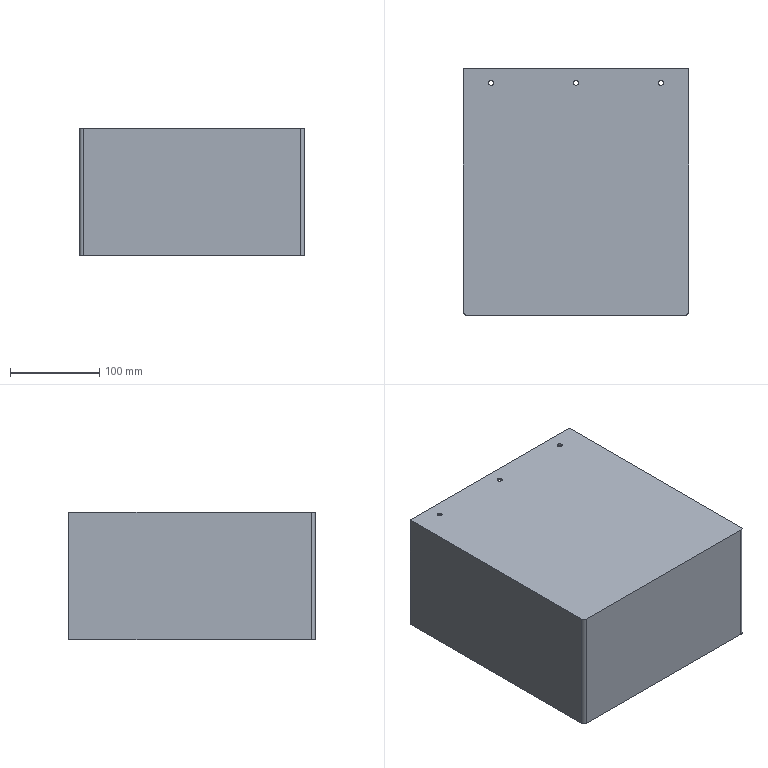Part | SolidWorks | features SMBaseFlange 3, SheetMetal 3, CombineBodies 1, Cut 1, Fillet 1, FlatPattern 1, HoleWzd 1 | 1 solid | 29 faces | box 252 x 276 x 143 mm | volume 499174 mm3 | cylinder 18 | plane 11 | commonest cylinder face diameters 5.5 x12 4 x2 8 x2 16.075 x2
STEP:
#1=CARTESIAN_POINT('',(124.,241.075,44.388));
#2=VERTEX_POINT('',#1);
#3=CARTESIAN_POINT('',(124.,257.15,44.388));
#4=VERTEX_POINT('',#3);
#5=CARTESIAN_POINT('',(124.,249.112,44.388));
#6=DIRECTION('',(1.,0.,0.));
#7=DIRECTION('',(0.,1.,0.));
#8=AXIS2_PLACEMENT_3D('',#5,#6,#7);
#9=CIRCLE('',#8,8.038);
#10=EDGE_CURVE('',#2,#4,#9,.T.);
#11=ORIENTED_EDGE('',*,*,#10,.F.);
#12=CARTESIAN_POINT('',(126.,241.075,44.388));
#13=VERTEX_POINT('',#12);
#14=CARTESIAN_POINT('',(116.,241.075,44.388));
#15=DIRECTION('',(1.,0.,0.));
#16=VECTOR('',#15,1000.);
#17=LINE('',#14,#16);
#18=EDGE_CURVE('',#2,#13,#17,.T.);
#19=ORIENTED_EDGE('',*,*,#18,.T.);
#20=CARTESIAN_POINT('',(126.,257.15,44.388));
#21=VERTEX_POINT('',#20);
#22=CARTESIAN_POINT('',(126.,249.112,44.388));
#23=DIRECTION('',(1.,0.,0.));
#24=DIRECTION('',(0.,1.,0.));
#25=AXIS2_PLACEMENT_3D('',#22,#23,#24);
#26=CIRCLE('',#25,8.038);
#27=EDGE_CURVE('',#13,#21,#26,.T.);
#28=ORIENTED_EDGE('',*,*,#27,.T.);
#29=CARTESIAN_POINT('',(116.,257.15,44.388));
#30=DIRECTION('',(1.,0.,0.));
#31=VECTOR('',#30,1000.);
#32=LINE('',#29,#31);
#33=EDGE_CURVE('',#4,#21,#32,.T.);
#34=ORIENTED_EDGE('',*,*,#33,.F.);
#35=EDGE_LOOP('',(#11,#19,#28,#34));
#36=FACE_OUTER_BOUND('',#35,.T.);
#37=CARTESIAN_POINT('',(116.,249.112,44.388));
#38=DIRECTION('',(1.,0.,0.));
#39=DIRECTION('',(0.,1.,0.));
#40=AXIS2_PLACEMENT_3D('',#37,#38,#39);
#41=CYLINDRICAL_SURFACE('',#40,8.038);
#42=ADVANCED_FACE('',(#36),#41,.F.);
#43=CARTESIAN_POINT('',(97.75,260.,71.5));
#44=VERTEX_POINT('',#43);
#45=CARTESIAN_POINT('',(92.25,260.,71.5));
#46=VERTEX_POINT('',#45);
#47=CARTESIAN_POINT('',(95.,260.,71.5));
#48=DIRECTION('',(0.,0.,-1.));
#49=DIRECTION('',(-1.,0.,0.));
#50=AXIS2_PLACEMENT_3D('',#47,#48,#49);
#51=CIRCLE('',#50,2.75);
#52=EDGE_CURVE('',#44,#46,#51,.T.);
#53=ORIENTED_EDGE('',*,*,#52,.F.);
#54=CARTESIAN_POINT('',(97.75,260.,69.5));
#55=VERTEX_POINT('',#54);
#56=CARTESIAN_POINT('',(97.75,260.,-71.5));
#57=DIRECTION('',(0.,0.,-1.));
#58=VECTOR('',#57,1000.);
#59=LINE('',#56,#58);
#60=EDGE_CURVE('',#44,#55,#59,.T.);
#61=ORIENTED_EDGE('',*,*,#60,.T.);
#62=CARTESIAN_POINT('',(92.25,260.,69.5));
#63=VERTEX_POINT('',#62);
#64=CARTESIAN_POINT('',(95.,260.,69.5));
#65=DIRECTION('',(0.,0.,1.));
#66=DIRECTION('',(1.,0.,0.));
#67=AXIS2_PLACEMENT_3D('',#64,#65,#66);
#68=CIRCLE('',#67,2.75);
#69=EDGE_CURVE('',#63,#55,#68,.T.);
#70=ORIENTED_EDGE('',*,*,#69,.F.);
#71=CARTESIAN_POINT('',(92.25,260.,-71.5));
#72=DIRECTION('',(0.,0.,-1.));
#73=VECTOR('',#72,1000.);
#74=LINE('',#71,#73);
#75=EDGE_CURVE('',#46,#63,#74,.T.);
#76=ORIENTED_EDGE('',*,*,#75,.F.);
#77=EDGE_LOOP('',(#53,#61,#70,#76));
#78=FACE_OUTER_BOUND('',#77,.T.);
#79=CARTESIAN_POINT('',(95.,260.,-71.5));
#80=DIRECTION('',(0.,0.,-1.));
#81=DIRECTION('',(-1.,0.,0.));
#82=AXIS2_PLACEMENT_3D('',#79,#80,#81);
#83=CYLINDRICAL_SURFACE('',#82,2.75);
#84=ADVANCED_FACE('',(#78),#83,.F.);
#85=CARTESIAN_POINT('',(2.75,260.,71.5));
#86=VERTEX_POINT('',#85);
#87=CARTESIAN_POINT('',(-2.75,260.,71.5));
#88=VERTEX_POINT('',#87);
#89=CARTESIAN_POINT('',(0.,260.,71.5));
#90=DIRECTION('',(0.,0.,-1.));
#91=DIRECTION('',(-1.,0.,0.));
#92=AXIS2_PLACEMENT_3D('',#89,#90,#91);
#93=CIRCLE('',#92,2.75);
#94=EDGE_CURVE('',#86,#88,#93,.T.);
#95=ORIENTED_EDGE('',*,*,#94,.F.);
#96=CARTESIAN_POINT('',(2.75,260.,69.5));
#97=VERTEX_POINT('',#96);
#98=CARTESIAN_POINT('',(2.75,260.,-71.5));
#99=DIRECTION('',(0.,0.,-1.));
#100=VECTOR('',#99,1000.);
#101=LINE('',#98,#100);
#102=EDGE_CURVE('',#86,#97,#101,.T.);
#103=ORIENTED_EDGE('',*,*,#102,.T.);
#104=CARTESIAN_POINT('',(-2.75,260.,69.5));
#105=VERTEX_POINT('',#104);
#106=CARTESIAN_POINT('',(0.,260.,69.5));
#107=DIRECTION('',(0.,0.,1.));
#108=DIRECTION('',(1.,0.,0.));
#109=AXIS2_PLACEMENT_3D('',#106,#107,#108);
#110=CIRCLE('',#109,2.75);
#111=EDGE_CURVE('',#105,#97,#110,.T.);
#112=ORIENTED_EDGE('',*,*,#111,.F.);
#113=CARTESIAN_POINT('',(-2.75,260.,-71.5));
#114=DIRECTION('',(0.,0.,-1.));
#115=VECTOR('',#114,1000.);
#116=LINE('',#113,#115);
#117=EDGE_CURVE('',#88,#105,#116,.T.);
#118=ORIENTED_EDGE('',*,*,#117,.F.);
#119=EDGE_LOOP('',(#95,#103,#112,#118));
#120=FACE_OUTER_BOUND('',#119,.T.);
#121=CARTESIAN_POINT('',(0.,260.,-71.5));
#122=DIRECTION('',(0.,0.,-1.));
#123=DIRECTION('',(-1.,0.,0.));
#124=AXIS2_PLACEMENT_3D('',#121,#122,#123);
#125=CYLINDRICAL_SURFACE('',#124,2.75);
#126=ADVANCED_FACE('',(#120),#125,.F.);
#127=CARTESIAN_POINT('',(-92.25,260.,71.5));
#128=VERTEX_POINT('',#127);
#129=CARTESIAN_POINT('',(-97.75,260.,71.5));
#130=VERTEX_POINT('',#129);
#131=CARTESIAN_POINT('',(-95.,260.,71.5));
#132=DIRECTION('',(0.,0.,-1.));
#133=DIRECTION('',(-1.,0.,0.));
#134=AXIS2_PLACEMENT_3D('',#131,#132,#133);
#135=CIRCLE('',#134,2.75);
#136=EDGE_CURVE('',#128,#130,#135,.T.);
#137=ORIENTED_EDGE('',*,*,#136,.F.);
#138=CARTESIAN_POINT('',(-92.25,260.,69.5));
#139=VERTEX_POINT('',#138);
#140=CARTESIAN_POINT('',(-92.25,260.,-71.5));
#141=DIRECTION('',(0.,0.,-1.));
#142=VECTOR('',#141,1000.);
#143=LINE('',#140,#142);
#144=EDGE_CURVE('',#128,#139,#143,.T.);
#145=ORIENTED_EDGE('',*,*,#144,.T.);
#146=CARTESIAN_POINT('',(-97.75,260.,69.5));
#147=VERTEX_POINT('',#146);
#148=CARTESIAN_POINT('',(-95.,260.,69.5));
#149=DIRECTION('',(0.,0.,1.));
#150=DIRECTION('',(1.,0.,0.));
#151=AXIS2_PLACEMENT_3D('',#148,#149,#150);
#152=CIRCLE('',#151,2.75);
#153=EDGE_CURVE('',#147,#139,#152,.T.);
#154=ORIENTED_EDGE('',*,*,#153,.F.);
#155=CARTESIAN_POINT('',(-97.75,260.,-71.5));
#156=DIRECTION('',(0.,0.,-1.));
#157=VECTOR('',#156,1000.);
#158=LINE('',#155,#157);
#159=EDGE_CURVE('',#130,#147,#158,.T.);
#160=ORIENTED_EDGE('',*,*,#159,.F.);
#161=EDGE_LOOP('',(#137,#145,#154,#160));
#162=FACE_OUTER_BOUND('',#161,.T.);
#163=CARTESIAN_POINT('',(-95.,260.,-71.5));
#164=DIRECTION('',(0.,0.,-1.));
#165=DIRECTION('',(-1.,0.,0.));
#166=AXIS2_PLACEMENT_3D('',#163,#164,#165);
#167=CYLINDRICAL_SURFACE('',#166,2.75);
#168=ADVANCED_FACE('',(#162),#167,.F.);
#169=CARTESIAN_POINT('',(97.75,260.,-69.5));
#170=VERTEX_POINT('',#169);
#171=CARTESIAN_POINT('',(92.25,260.,-69.5));
#172=VERTEX_POINT('',#171);
#173=CARTESIAN_POINT('',(95.,260.,-69.5));
#174=DIRECTION('',(0.,0.,-1.));
#175=DIRECTION('',(-1.,0.,0.));
#176=AXIS2_PLACEMENT_3D('',#173,#174,#175);
#177=CIRCLE('',#176,2.75);
#178=EDGE_CURVE('',#170,#172,#177,.T.);
#179=ORIENTED_EDGE('',*,*,#178,.F.);
#180=CARTESIAN_POINT('',(97.75,260.,-71.5));
#181=VERTEX_POINT('',#180);
#182=CARTESIAN_POINT('',(97.75,260.,-71.5));
#183=DIRECTION('',(0.,0.,-1.));
#184=VECTOR('',#183,1000.);
#185=LINE('',#182,#184);
#186=EDGE_CURVE('',#170,#181,#185,.T.);
#187=ORIENTED_EDGE('',*,*,#186,.T.);
#188=CARTESIAN_POINT('',(92.25,260.,-71.5));
#189=VERTEX_POINT('',#188);
#190=CARTESIAN_POINT('',(95.,260.,-71.5));
#191=DIRECTION('',(0.,0.,-1.));
#192=DIRECTION('',(-1.,0.,0.));
#193=AXIS2_PLACEMENT_3D('',#190,#191,#192);
#194=CIRCLE('',#193,2.75);
#195=EDGE_CURVE('',#181,#189,#194,.T.);
#196=ORIENTED_EDGE('',*,*,#195,.T.);
#197=CARTESIAN_POINT('',(92.25,260.,-71.5));
#198=DIRECTION('',(0.,0.,-1.));
#199=VECTOR('',#198,1000.);
#200=LINE('',#197,#199);
#201=EDGE_CURVE('',#172,#189,#200,.T.);
#202=ORIENTED_EDGE('',*,*,#201,.F.);
#203=EDGE_LOOP('',(#179,#187,#196,#202));
#204=FACE_OUTER_BOUND('',#203,.T.);
#205=CARTESIAN_POINT('',(95.,260.,-71.5));
#206=DIRECTION('',(0.,0.,-1.));
#207=DIRECTION('',(-1.,0.,0.));
#208=AXIS2_PLACEMENT_3D('',#205,#206,#207);
#209=CYLINDRICAL_SURFACE('',#208,2.75);
#210=ADVANCED_FACE('',(#204),#209,.F.);
#211=CARTESIAN_POINT('',(2.75,260.,-69.5));
#212=VERTEX_POINT('',#211);
#213=CARTESIAN_POINT('',(-2.75,260.,-69.5));
#214=VERTEX_POINT('',#213);
#215=CARTESIAN_POINT('',(0.,260.,-69.5));
#216=DIRECTION('',(0.,0.,-1.));
#217=DIRECTION('',(-1.,0.,0.));
#218=AXIS2_PLACEMENT_3D('',#215,#216,#217);
#219=CIRCLE('',#218,2.75);
#220=EDGE_CURVE('',#212,#214,#219,.T.);
#221=ORIENTED_EDGE('',*,*,#220,.F.);
#222=CARTESIAN_POINT('',(2.75,260.,-71.5));
#223=VERTEX_POINT('',#222);
#224=CARTESIAN_POINT('',(2.75,260.,-71.5));
#225=DIRECTION('',(0.,0.,-1.));
#226=VECTOR('',#225,1000.);
#227=LINE('',#224,#226);
#228=EDGE_CURVE('',#212,#223,#227,.T.);
#229=ORIENTED_EDGE('',*,*,#228,.T.);
#230=CARTESIAN_POINT('',(-2.75,260.,-71.5));
#231=VERTEX_POINT('',#230);
#232=CARTESIAN_POINT('',(0.,260.,-71.5));
#233=DIRECTION('',(0.,0.,-1.));
#234=DIRECTION('',(-1.,0.,0.));
#235=AXIS2_PLACEMENT_3D('',#232,#233,#234);
#236=CIRCLE('',#235,2.75);
#237=EDGE_CURVE('',#223,#231,#236,.T.);
#238=ORIENTED_EDGE('',*,*,#237,.T.);
#239=CARTESIAN_POINT('',(-2.75,260.,-71.5));
#240=DIRECTION('',(0.,0.,-1.));
#241=VECTOR('',#240,1000.);
#242=LINE('',#239,#241);
#243=EDGE_CURVE('',#214,#231,#242,.T.);
#244=ORIENTED_EDGE('',*,*,#243,.F.);
#245=EDGE_LOOP('',(#221,#229,#238,#244));
#246=FACE_OUTER_BOUND('',#245,.T.);
#247=CARTESIAN_POINT('',(0.,260.,-71.5));
#248=DIRECTION('',(0.,0.,-1.));
#249=DIRECTION('',(-1.,0.,0.));
#250=AXIS2_PLACEMENT_3D('',#247,#248,#249);
#251=CYLINDRICAL_SURFACE('',#250,2.75);
#252=ADVANCED_FACE('',(#246),#251,.F.);
#253=CARTESIAN_POINT('',(-92.25,260.,-69.5));
#254=VERTEX_POINT('',#253);
#255=CARTESIAN_POINT('',(-97.75,260.,-69.5));
#256=VERTEX_POINT('',#255);
#257=CARTESIAN_POINT('',(-95.,260.,-69.5));
#258=DIRECTION('',(0.,0.,-1.));
#259=DIRECTION('',(-1.,0.,0.));
#260=AXIS2_PLACEMENT_3D('',#257,#258,#259);
#261=CIRCLE('',#260,2.75);
#262=EDGE_CURVE('',#254,#256,#261,.T.);
#263=ORIENTED_EDGE('',*,*,#262,.F.);
#264=CARTESIAN_POINT('',(-92.25,260.,-71.5));
#265=VERTEX_POINT('',#264);
#266=CARTESIAN_POINT('',(-92.25,260.,-71.5));
#267=DIRECTION('',(0.,0.,-1.));
#268=VECTOR('',#267,1000.);
#269=LINE('',#266,#268);
#270=EDGE_CURVE('',#254,#265,#269,.T.);
#271=ORIENTED_EDGE('',*,*,#270,.T.);
#272=CARTESIAN_POINT('',(-97.75,260.,-71.5));
#273=VERTEX_POINT('',#272);
#274=CARTESIAN_POINT('',(-95.,260.,-71.5));
#275=DIRECTION('',(0.,0.,-1.));
#276=DIRECTION('',(-1.,0.,0.));
#277=AXIS2_PLACEMENT_3D('',#274,#275,#276);
#278=CIRCLE('',#277,2.75);
#279=EDGE_CURVE('',#265,#273,#278,.T.);
#280=ORIENTED_EDGE('',*,*,#279,.T.);
#281=CARTESIAN_POINT('',(-97.75,260.,-71.5));
#282=DIRECTION('',(0.,0.,-1.));
#283=VECTOR('',#282,1000.);
#284=LINE('',#281,#283);
#285=EDGE_CURVE('',#256,#273,#284,.T.);
#286=ORIENTED_EDGE('',*,*,#285,.F.);
#287=EDGE_LOOP('',(#263,#271,#280,#286));
#288=FACE_OUTER_BOUND('',#287,.T.);
#289=CARTESIAN_POINT('',(-95.,260.,-71.5));
#290=DIRECTION('',(0.,0.,-1.));
#291=DIRECTION('',(-1.,0.,0.));
#292=AXIS2_PLACEMENT_3D('',#289,#290,#291);
#293=CYLINDRICAL_SURFACE('',#292,2.75);
#294=ADVANCED_FACE('',(#288),#293,.F.);
#295=CARTESIAN_POINT('',(-124.,4.,-69.5));
#296=VERTEX_POINT('',#295);
#297=CARTESIAN_POINT('',(-124.,276.,-69.5));
#298=VERTEX_POINT('',#297);
#299=CARTESIAN_POINT('',(-124.,276.,-69.5));
#300=DIRECTION('',(0.,1.,0.));
#301=VECTOR('',#300,1000.);
#302=LINE('',#299,#301);
#303=EDGE_CURVE('',#296,#298,#302,.T.);
#304=ORIENTED_EDGE('',*,*,#303,.T.);
#305=CARTESIAN_POINT('',(-124.,276.,69.5));
#306=VERTEX_POINT('',#305);
#307=CARTESIAN_POINT('',(-124.,276.,69.5));
#308=DIRECTION('',(0.,0.,-1.));
#309=VECTOR('',#308,1000.);
#310=LINE('',#307,#309);
#311=EDGE_CURVE('',#306,#298,#310,.T.);
#312=ORIENTED_EDGE('',*,*,#311,.F.);
#313=CARTESIAN_POINT('',(-124.,4.,69.5));
#314=VERTEX_POINT('',#313);
#315=CARTESIAN_POINT('',(-124.,276.,69.5));
#316=DIRECTION('',(0.,1.,0.));
#317=VECTOR('',#316,1000.);
#318=LINE('',#315,#317);
#319=EDGE_CURVE('',#314,#306,#318,.T.);
#320=ORIENTED_EDGE('',*,*,#319,.F.);
#321=CARTESIAN_POINT('',(-124.,4.,69.5));
#322=DIRECTION('',(0.,0.,-1.));
#323=VECTOR('',#322,1000.);
#324=LINE('',#321,#323);
#325=EDGE_CURVE('',#314,#296,#324,.T.);
#326=ORIENTED_EDGE('',*,*,#325,.T.);
#327=EDGE_LOOP('',(#304,#312,#320,#326));
#328=FACE_OUTER_BOUND('',#327,.T.);
#329=CARTESIAN_POINT('',(-124.,276.,69.5));
#330=DIRECTION('',(-1.,0.,0.));
#331=DIRECTION('',(0.,-1.,0.));
#332=AXIS2_PLACEMENT_3D('',#329,#330,#331);
#333=PLANE('',#332);
#334=ADVANCED_FACE('',(#328),#333,.F.);
#335=CARTESIAN_POINT('',(-126.,276.,71.5));
#336=VERTEX_POINT('',#335);
#337=CARTESIAN_POINT('',(-126.,276.,-71.5));
#338=VERTEX_POINT('',#337);
#339=CARTESIAN_POINT('',(-126.,276.,69.5));
#340=DIRECTION('',(0.,0.,-1.));
#341=VECTOR('',#340,1000.);
#342=LINE('',#339,#341);
#343=EDGE_CURVE('',#336,#338,#342,.T.);
#344=ORIENTED_EDGE('',*,*,#343,.T.);
#345=CARTESIAN_POINT('',(-126.,4.,-71.5));
#346=VERTEX_POINT('',#345);
#347=CARTESIAN_POINT('',(-126.,4.,-71.5));
#348=DIRECTION('',(0.,1.,0.));
#349=VECTOR('',#348,1000.);
#350=LINE('',#347,#349);
#351=EDGE_CURVE('',#346,#338,#350,.T.);
#352=ORIENTED_EDGE('',*,*,#351,.F.);
#353=CARTESIAN_POINT('',(-126.,4.,71.5));
#354=VERTEX_POINT('',#353);
#355=CARTESIAN_POINT('',(-126.,4.,69.5));
#356=DIRECTION('',(0.,0.,-1.));
#357=VECTOR('',#356,1000.);
#358=LINE('',#355,#357);
#359=EDGE_CURVE('',#354,#346,#358,.T.);
#360=ORIENTED_EDGE('',*,*,#359,.F.);
#361=CARTESIAN_POINT('',(-126.,276.,71.5));
#362=DIRECTION('',(0.,-1.,0.));
#363=VECTOR('',#362,1000.);
#364=LINE('',#361,#363);
#365=EDGE_CURVE('',#336,#354,#364,.T.);
#366=ORIENTED_EDGE('',*,*,#365,.F.);
#367=EDGE_LOOP('',(#344,#352,#360,#366));
#368=FACE_OUTER_BOUND('',#367,.T.);
#369=CARTESIAN_POINT('',(-126.,276.,69.5));
#370=DIRECTION('',(-1.,0.,0.));
#371=DIRECTION('',(0.,-1.,0.));
#372=AXIS2_PLACEMENT_3D('',#369,#370,#371);
#373=PLANE('',#372);
#374=ADVANCED_FACE('',(#368),#373,.T.);
#375=ORIENTED_EDGE('',*,*,#359,.T.);
#376=CARTESIAN_POINT('',(-122.,0.,-71.5));
#377=VERTEX_POINT('',#376);
#378=CARTESIAN_POINT('',(-122.,4.,-71.5));
#379=DIRECTION('',(0.,0.,-1.));
#380=DIRECTION('',(-1.,0.,0.));
#381=AXIS2_PLACEMENT_3D('',#378,#379,#380);
#382=CIRCLE('',#381,4.);
#383=EDGE_CURVE('',#377,#346,#382,.T.);
#384=ORIENTED_EDGE('',*,*,#383,.F.);
#385=CARTESIAN_POINT('',(-122.,0.,71.5));
#386=VERTEX_POINT('',#385);
#387=CARTESIAN_POINT('',(-122.,0.,69.5));
#388=DIRECTION('',(0.,0.,-1.));
#389=VECTOR('',#388,1000.);
#390=LINE('',#387,#389);
#391=EDGE_CURVE('',#386,#377,#390,.T.);
#392=ORIENTED_EDGE('',*,*,#391,.F.);
#393=CARTESIAN_POINT('',(-122.,4.,71.5));
#394=DIRECTION('',(0.,0.,1.));
#395=DIRECTION('',(1.,0.,0.));
#396=AXIS2_PLACEMENT_3D('',#393,#394,#395);
#397=CIRCLE('',#396,4.);
#398=EDGE_CURVE('',#354,#386,#397,.T.);
#399=ORIENTED_EDGE('',*,*,#398,.F.);
#400=EDGE_LOOP('',(#375,#384,#392,#399));
#401=FACE_OUTER_BOUND('',#400,.T.);
#402=CARTESIAN_POINT('',(-122.,4.,69.5));
#403=DIRECTION('',(0.,0.,-1.));
#404=DIRECTION('',(-1.,0.,0.));
#405=AXIS2_PLACEMENT_3D('',#402,#403,#404);
#406=CYLINDRICAL_SURFACE('',#405,4.);
#407=ADVANCED_FACE('',(#401),#406,.T.);
#408=ORIENTED_EDGE('',*,*,#391,.T.);
#409=CARTESIAN_POINT('',(122.,0.,-71.5));
#410=VERTEX_POINT('',#409);
#411=CARTESIAN_POINT('',(122.,0.,-71.5));
#412=DIRECTION('',(-1.,0.,0.));
#413=VECTOR('',#412,1000.);
#414=LINE('',#411,#413);
#415=EDGE_CURVE('',#410,#377,#414,.T.);
#416=ORIENTED_EDGE('',*,*,#415,.F.);
#417=CARTESIAN_POINT('',(122.,0.,71.5));
#418=VERTEX_POINT('',#417);
#419=CARTESIAN_POINT('',(122.,0.,69.5));
#420=DIRECTION('',(0.,0.,-1.));
#421=VECTOR('',#420,1000.);
#422=LINE('',#419,#421);
#423=EDGE_CURVE('',#418,#410,#422,.T.);
#424=ORIENTED_EDGE('',*,*,#423,.F.);
#425=CARTESIAN_POINT('',(-126.,0.,71.5));
#426=DIRECTION('',(1.,0.,0.));
#427=VECTOR('',#426,1000.);
#428=LINE('',#425,#427);
#429=EDGE_CURVE('',#386,#418,#428,.T.);
#430=ORIENTED_EDGE('',*,*,#429,.F.);
#431=EDGE_LOOP('',(#408,#416,#424,#430));
#432=FACE_OUTER_BOUND('',#431,.T.);
#433=CARTESIAN_POINT('',(-126.,0.,69.5));
#434=DIRECTION('',(0.,-1.,0.));
#435=DIRECTION('',(0.,0.,-1.));
#436=AXIS2_PLACEMENT_3D('',#433,#434,#435);
#437=PLANE('',#436);
#438=ADVANCED_FACE('',(#432),#437,.T.);
#439=ORIENTED_EDGE('',*,*,#423,.T.);
#440=CARTESIAN_POINT('',(126.,4.,-71.5));
#441=VERTEX_POINT('',#440);
#442=CARTESIAN_POINT('',(122.,4.,-71.5));
#443=DIRECTION('',(0.,0.,-1.));
#444=DIRECTION('',(-1.,0.,0.));
#445=AXIS2_PLACEMENT_3D('',#442,#443,#444);
#446=CIRCLE('',#445,4.);
#447=EDGE_CURVE('',#441,#410,#446,.T.);
#448=ORIENTED_EDGE('',*,*,#447,.F.);
#449=CARTESIAN_POINT('',(126.,4.,71.5));
#450=VERTEX_POINT('',#449);
#451=CARTESIAN_POINT('',(126.,4.,69.5));
#452=DIRECTION('',(0.,0.,-1.));
#453=VECTOR('',#452,1000.);
#454=LINE('',#451,#453);
#455=EDGE_CURVE('',#450,#441,#454,.T.);
#456=ORIENTED_EDGE('',*,*,#455,.F.);
#457=CARTESIAN_POINT('',(122.,4.,71.5));
#458=DIRECTION('',(0.,0.,1.));
#459=DIRECTION('',(1.,0.,0.));
#460=AXIS2_PLACEMENT_3D('',#457,#458,#459);
#461=CIRCLE('',#460,4.);
#462=EDGE_CURVE('',#418,#450,#461,.T.);
#463=ORIENTED_EDGE('',*,*,#462,.F.);
#464=EDGE_LOOP('',(#439,#448,#456,#463));
#465=FACE_OUTER_BOUND('',#464,.T.);
#466=CARTESIAN_POINT('',(122.,4.,69.5));
#467=DIRECTION('',(0.,0.,-1.));
#468=DIRECTION('',(-1.,0.,0.));
#469=AXIS2_PLACEMENT_3D('',#466,#467,#468);
#470=CYLINDRICAL_SURFACE('',#469,4.);
#471=ADVANCED_FACE('',(#465),#470,.T.);
#472=CARTESIAN_POINT('',(126.,249.112,44.388));
#473=DIRECTION('',(1.,0.,0.));
#474=DIRECTION('',(0.,1.,0.));
#475=AXIS2_PLACEMENT_3D('',#472,#473,#474);
#476=CIRCLE('',#475,8.038);
#477=EDGE_CURVE('',#21,#13,#476,.T.);
#478=ORIENTED_EDGE('',*,*,#477,.F.);
#479=ORIENTED_EDGE('',*,*,#27,.F.);
#480=EDGE_LOOP('',(#478,#479));
#481=FACE_BOUND('',#480,.T.);
#482=ORIENTED_EDGE('',*,*,#455,.T.);
#483=CARTESIAN_POINT('',(126.,276.,-71.5));
#484=VERTEX_POINT('',#483);
#485=CARTESIAN_POINT('',(126.,276.,-71.5));
#486=DIRECTION('',(0.,-1.,0.));
#487=VECTOR('',#486,1000.);
#488=LINE('',#485,#487);
#489=EDGE_CURVE('',#484,#441,#488,.T.);
#490=ORIENTED_EDGE('',*,*,#489,.F.);
#491=CARTESIAN_POINT('',(126.,276.,71.5));
#492=VERTEX_POINT('',#491);
#493=CARTESIAN_POINT('',(126.,276.,69.5));
#494=DIRECTION('',(0.,0.,-1.));
#495=VECTOR('',#494,1000.);
#496=LINE('',#493,#495);
#497=EDGE_CURVE('',#492,#484,#496,.T.);
#498=ORIENTED_EDGE('',*,*,#497,.F.);
#499=CARTESIAN_POINT('',(126.,276.,71.5));
#500=DIRECTION('',(0.,1.,0.));
#501=VECTOR('',#500,1000.);
#502=LINE('',#499,#501);
#503=EDGE_CURVE('',#450,#492,#502,.T.);
#504=ORIENTED_EDGE('',*,*,#503,.F.);
#505=EDGE_LOOP('',(#482,#490,#498,#504));
#506=FACE_OUTER_BOUND('',#505,.T.);
#507=CARTESIAN_POINT('',(126.,276.,69.5));
#508=DIRECTION('',(1.,0.,0.));
#509=DIRECTION('',(0.,1.,0.));
#510=AXIS2_PLACEMENT_3D('',#507,#508,#509);
#511=PLANE('',#510);
#512=ADVANCED_FACE('',(#481,#506),#511,.T.);
#513=CARTESIAN_POINT('',(124.,276.,69.5));
#514=VERTEX_POINT('',#513);
#515=CARTESIAN_POINT('',(-126.,276.,69.5));
#516=DIRECTION('',(-1.,0.,0.));
#517=VECTOR('',#516,1000.);
#518=LINE('',#515,#517);
#519=EDGE_CURVE('',#514,#306,#518,.T.);
#520=ORIENTED_EDGE('',*,*,#519,.T.);
#521=ORIENTED_EDGE('',*,*,#311,.T.);
#522=CARTESIAN_POINT('',(124.,276.,-69.5));
#523=VERTEX_POINT('',#522);
#524=CARTESIAN_POINT('',(-126.,276.,-69.5));
#525=DIRECTION('',(1.,0.,0.));
#526=VECTOR('',#525,1000.);
#527=LINE('',#524,#526);
#528=EDGE_CURVE('',#298,#523,#527,.T.);
#529=ORIENTED_EDGE('',*,*,#528,.T.);
#530=CARTESIAN_POINT('',(124.,276.,69.5));
#531=DIRECTION('',(0.,0.,-1.));
#532=VECTOR('',#531,1000.);
#533=LINE('',#530,#532);
#534=EDGE_CURVE('',#514,#523,#533,.T.);
#535=ORIENTED_EDGE('',*,*,#534,.F.);
#536=EDGE_LOOP('',(#520,#521,#529,#535));
#537=FACE_BOUND('',#536,.T.);
#538=ORIENTED_EDGE('',*,*,#497,.T.);
#539=CARTESIAN_POINT('',(-126.,276.,-71.5));
#540=DIRECTION('',(1.,0.,0.));
#541=VECTOR('',#540,1000.);
#542=LINE('',#539,#541);
#543=EDGE_CURVE('',#338,#484,#542,.T.);
#544=ORIENTED_EDGE('',*,*,#543,.F.);
#545=ORIENTED_EDGE('',*,*,#343,.F.);
#546=CARTESIAN_POINT('',(-126.,276.,71.5));
#547=DIRECTION('',(-1.,0.,0.));
#548=VECTOR('',#547,1000.);
#549=LINE('',#546,#548);
#550=EDGE_CURVE('',#492,#336,#549,.T.);
#551=ORIENTED_EDGE('',*,*,#550,.F.);
#552=EDGE_LOOP('',(#538,#544,#545,#551));
#553=FACE_OUTER_BOUND('',#552,.T.);
#554=CARTESIAN_POINT('',(124.,276.,69.5));
#555=DIRECTION('',(0.,1.,0.));
#556=DIRECTION('',(0.,0.,1.));
#557=AXIS2_PLACEMENT_3D('',#554,#555,#556);
#558=PLANE('',#557);
#559=ADVANCED_FACE('',(#537,#553),#558,.T.);
#560=CARTESIAN_POINT('',(124.,249.112,44.388));
#561=DIRECTION('',(1.,0.,0.));
#562=DIRECTION('',(0.,1.,0.));
#563=AXIS2_PLACEMENT_3D('',#560,#561,#562);
#564=CIRCLE('',#563,8.038);
#565=EDGE_CURVE('',#4,#2,#564,.T.);
#566=ORIENTED_EDGE('',*,*,#565,.T.);
#567=ORIENTED_EDGE('',*,*,#10,.T.);
#568=EDGE_LOOP('',(#566,#567));
#569=FACE_BOUND('',#568,.T.);
#570=CARTESIAN_POINT('',(124.,4.,-69.5));
#571=VERTEX_POINT('',#570);
#572=CARTESIAN_POINT('',(124.,276.,-69.5));
#573=DIRECTION('',(0.,-1.,0.));
#574=VECTOR('',#573,1000.);
#575=LINE('',#572,#574);
#576=EDGE_CURVE('',#523,#571,#575,.T.);
#577=ORIENTED_EDGE('',*,*,#576,.T.);
#578=CARTESIAN_POINT('',(124.,4.,69.5));
#579=VERTEX_POINT('',#578);
#580=CARTESIAN_POINT('',(124.,4.,69.5));
#581=DIRECTION('',(0.,0.,-1.));
#582=VECTOR('',#581,1000.);
#583=LINE('',#580,#582);
#584=EDGE_CURVE('',#579,#571,#583,.T.);
#585=ORIENTED_EDGE('',*,*,#584,.F.);
#586=CARTESIAN_POINT('',(124.,276.,69.5));
#587=DIRECTION('',(0.,-1.,0.));
#588=VECTOR('',#587,1000.);
#589=LINE('',#586,#588);
#590=EDGE_CURVE('',#514,#579,#589,.T.);
#591=ORIENTED_EDGE('',*,*,#590,.F.);
#592=ORIENTED_EDGE('',*,*,#534,.T.);
#593=EDGE_LOOP('',(#577,#585,#591,#592));
#594=FACE_OUTER_BOUND('',#593,.T.);
#595=CARTESIAN_POINT('',(124.,276.,69.5));
#596=DIRECTION('',(1.,0.,0.));
#597=DIRECTION('',(0.,1.,0.));
#598=AXIS2_PLACEMENT_3D('',#595,#596,#597);
#599=PLANE('',#598);
#600=ADVANCED_FACE('',(#569,#594),#599,.F.);
#601=CARTESIAN_POINT('',(122.,2.,-69.5));
#602=VERTEX_POINT('',#601);
#603=CARTESIAN_POINT('',(122.,4.,-69.5));
#604=DIRECTION('',(0.,0.,-1.));
#605=DIRECTION('',(1.,0.,0.));
#606=AXIS2_PLACEMENT_3D('',#603,#604,#605);
#607=CIRCLE('',#606,2.);
#608=EDGE_CURVE('',#571,#602,#607,.T.);
#609=ORIENTED_EDGE('',*,*,#608,.T.);
#610=CARTESIAN_POINT('',(122.,2.,69.5));
#611=VERTEX_POINT('',#610);
#612=CARTESIAN_POINT('',(122.,2.,69.5));
#613=DIRECTION('',(0.,0.,-1.));
#614=VECTOR('',#613,1000.);
#615=LINE('',#612,#614);
#616=EDGE_CURVE('',#611,#602,#615,.T.);
#617=ORIENTED_EDGE('',*,*,#616,.F.);
#618=CARTESIAN_POINT('',(122.,4.,69.5));
#619=DIRECTION('',(0.,0.,-1.));
#620=DIRECTION('',(1.,0.,0.));
#621=AXIS2_PLACEMENT_3D('',#618,#619,#620);
#622=CIRCLE('',#621,2.);
#623=EDGE_CURVE('',#579,#611,#622,.T.);
#624=ORIENTED_EDGE('',*,*,#623,.F.);
#625=ORIENTED_EDGE('',*,*,#584,.T.);
#626=EDGE_LOOP('',(#609,#617,#624,#625));
#627=FACE_OUTER_BOUND('',#626,.T.);
#628=CARTESIAN_POINT('',(122.,4.,69.5));
#629=DIRECTION('',(0.,0.,-1.));
#630=DIRECTION('',(-1.,0.,0.));
#631=AXIS2_PLACEMENT_3D('',#628,#629,#630);
#632=CYLINDRICAL_SURFACE('',#631,2.);
#633=ADVANCED_FACE('',(#627),#632,.F.);
#634=CARTESIAN_POINT('',(-122.,2.,-69.5));
#635=VERTEX_POINT('',#634);
#636=CARTESIAN_POINT('',(-126.,2.,-69.5));
#637=DIRECTION('',(-1.,0.,0.));
#638=VECTOR('',#637,1000.);
#639=LINE('',#636,#638);
#640=EDGE_CURVE('',#602,#635,#639,.T.);
#641=ORIENTED_EDGE('',*,*,#640,.T.);
#642=CARTESIAN_POINT('',(-122.,2.,69.5));
#643=VERTEX_POINT('',#642);
#644=CARTESIAN_POINT('',(-122.,2.,69.5));
#645=DIRECTION('',(0.,0.,-1.));
#646=VECTOR('',#645,1000.);
#647=LINE('',#644,#646);
#648=EDGE_CURVE('',#643,#635,#647,.T.);
#649=ORIENTED_EDGE('',*,*,#648,.F.);
#650=CARTESIAN_POINT('',(-126.,2.,69.5));
#651=DIRECTION('',(-1.,0.,0.));
#652=VECTOR('',#651,1000.);
#653=LINE('',#650,#652);
#654=EDGE_CURVE('',#611,#643,#653,.T.);
#655=ORIENTED_EDGE('',*,*,#654,.F.);
#656=ORIENTED_EDGE('',*,*,#616,.T.);
#657=EDGE_LOOP('',(#641,#649,#655,#656));
#658=FACE_OUTER_BOUND('',#657,.T.);
#659=CARTESIAN_POINT('',(-126.,2.,69.5));
#660=DIRECTION('',(0.,-1.,0.));
#661=DIRECTION('',(0.,0.,-1.));
#662=AXIS2_PLACEMENT_3D('',#659,#660,#661);
#663=PLANE('',#662);
#664=ADVANCED_FACE('',(#658),#663,.F.);
#665=CARTESIAN_POINT('',(-122.,4.,-69.5));
#666=DIRECTION('',(0.,0.,-1.));
#667=DIRECTION('',(1.,0.,0.));
#668=AXIS2_PLACEMENT_3D('',#665,#666,#667);
#669=CIRCLE('',#668,2.);
#670=EDGE_CURVE('',#635,#296,#669,.T.);
#671=ORIENTED_EDGE('',*,*,#670,.T.);
#672=ORIENTED_EDGE('',*,*,#325,.F.);
#673=CARTESIAN_POINT('',(-122.,4.,69.5));
#674=DIRECTION('',(0.,0.,-1.));
#675=DIRECTION('',(1.,0.,0.));
#676=AXIS2_PLACEMENT_3D('',#673,#674,#675);
#677=CIRCLE('',#676,2.);
#678=EDGE_CURVE('',#643,#314,#677,.T.);
#679=ORIENTED_EDGE('',*,*,#678,.F.);
#680=ORIENTED_EDGE('',*,*,#648,.T.);
#681=EDGE_LOOP('',(#671,#672,#679,#680));
#682=FACE_OUTER_BOUND('',#681,.T.);
#683=CARTESIAN_POINT('',(-122.,4.,69.5));
#684=DIRECTION('',(0.,0.,-1.));
#685=DIRECTION('',(-1.,0.,0.));
#686=AXIS2_PLACEMENT_3D('',#683,#684,#685);
#687=CYLINDRICAL_SURFACE('',#686,2.);
#688=ADVANCED_FACE('',(#682),#687,.F.);
#689=CARTESIAN_POINT('',(95.,260.,-71.5));
#690=DIRECTION('',(0.,0.,-1.));
#691=DIRECTION('',(-1.,0.,0.));
#692=AXIS2_PLACEMENT_3D('',#689,#690,#691);
#693=CIRCLE('',#692,2.75);
#694=EDGE_CURVE('',#189,#181,#693,.T.);
#695=ORIENTED_EDGE('',*,*,#694,.F.);
#696=ORIENTED_EDGE('',*,*,#195,.F.);
#697=EDGE_LOOP('',(#695,#696));
#698=FACE_BOUND('',#697,.T.);
#699=CARTESIAN_POINT('',(0.,260.,-71.5));
#700=DIRECTION('',(0.,0.,-1.));
#701=DIRECTION('',(-1.,0.,0.));
#702=AXIS2_PLACEMENT_3D('',#699,#700,#701);
#703=CIRCLE('',#702,2.75);
#704=EDGE_CURVE('',#231,#223,#703,.T.);
#705=ORIENTED_EDGE('',*,*,#704,.F.);
#706=ORIENTED_EDGE('',*,*,#237,.F.);
#707=EDGE_LOOP('',(#705,#706));
#708=FACE_BOUND('',#707,.T.);
#709=CARTESIAN_POINT('',(-95.,260.,-71.5));
#710=DIRECTION('',(0.,0.,-1.));
#711=DIRECTION('',(-1.,0.,0.));
#712=AXIS2_PLACEMENT_3D('',#709,#710,#711);
#713=CIRCLE('',#712,2.75);
#714=EDGE_CURVE('',#273,#265,#713,.T.);
#715=ORIENTED_EDGE('',*,*,#714,.F.);
#716=ORIENTED_EDGE('',*,*,#279,.F.);
#717=EDGE_LOOP('',(#715,#716));
#718=FACE_BOUND('',#717,.T.);
#719=ORIENTED_EDGE('',*,*,#543,.T.);
#720=ORIENTED_EDGE('',*,*,#489,.T.);
#721=ORIENTED_EDGE('',*,*,#447,.T.);
#722=ORIENTED_EDGE('',*,*,#415,.T.);
#723=ORIENTED_EDGE('',*,*,#383,.T.);
#724=ORIENTED_EDGE('',*,*,#351,.T.);
#725=EDGE_LOOP('',(#719,#720,#721,#722,#723,#724));
#726=FACE_OUTER_BOUND('',#725,.T.);
#727=CARTESIAN_POINT('',(122.,4.,-71.5));
#728=DIRECTION('',(0.,0.,-1.));
#729=DIRECTION('',(-1.,0.,0.));
#730=AXIS2_PLACEMENT_3D('',#727,#728,#729);
#731=PLANE('',#730);
#732=ADVANCED_FACE('',(#698,#708,#718,#726),#731,.T.);
#733=ORIENTED_EDGE('',*,*,#576,.F.);
#734=ORIENTED_EDGE('',*,*,#528,.F.);
#735=ORIENTED_EDGE('',*,*,#303,.F.);
#736=ORIENTED_EDGE('',*,*,#670,.F.);
#737=ORIENTED_EDGE('',*,*,#640,.F.);
#738=ORIENTED_EDGE('',*,*,#608,.F.);
#739=EDGE_LOOP('',(#733,#734,#735,#736,#737,#738));
#740=FACE_OUTER_BOUND('',#739,.T.);
#741=CARTESIAN_POINT('',(95.,260.,-69.5));
#742=DIRECTION('',(0.,0.,-1.));
#743=DIRECTION('',(-1.,0.,0.));
#744=AXIS2_PLACEMENT_3D('',#741,#742,#743);
#745=CIRCLE('',#744,2.75);
#746=EDGE_CURVE('',#172,#170,#745,.T.);
#747=ORIENTED_EDGE('',*,*,#746,.T.);
#748=ORIENTED_EDGE('',*,*,#178,.T.);
#749=EDGE_LOOP('',(#747,#748));
#750=FACE_BOUND('',#749,.T.);
#751=CARTESIAN_POINT('',(0.,260.,-69.5));
#752=DIRECTION('',(0.,0.,-1.));
#753=DIRECTION('',(-1.,0.,0.));
#754=AXIS2_PLACEMENT_3D('',#751,#752,#753);
#755=CIRCLE('',#754,2.75);
#756=EDGE_CURVE('',#214,#212,#755,.T.);
#757=ORIENTED_EDGE('',*,*,#756,.T.);
#758=ORIENTED_EDGE('',*,*,#220,.T.);
#759=EDGE_LOOP('',(#757,#758));
#760=FACE_BOUND('',#759,.T.);
#761=CARTESIAN_POINT('',(-95.,260.,-69.5));
#762=DIRECTION('',(0.,0.,-1.));
#763=DIRECTION('',(-1.,0.,0.));
#764=AXIS2_PLACEMENT_3D('',#761,#762,#763);
#765=CIRCLE('',#764,2.75);
#766=EDGE_CURVE('',#256,#254,#765,.T.);
#767=ORIENTED_EDGE('',*,*,#766,.T.);
#768=ORIENTED_EDGE('',*,*,#262,.T.);
#769=EDGE_LOOP('',(#767,#768));
#770=FACE_BOUND('',#769,.T.);
#771=CARTESIAN_POINT('',(122.,4.,-69.5));
#772=DIRECTION('',(0.,0.,-1.));
#773=DIRECTION('',(-1.,0.,0.));
#774=AXIS2_PLACEMENT_3D('',#771,#772,#773);
#775=PLANE('',#774);
#776=ADVANCED_FACE('',(#740,#750,#760,#770),#775,.F.);
#777=ORIENTED_EDGE('',*,*,#270,.F.);
#778=ORIENTED_EDGE('',*,*,#766,.F.);
#779=ORIENTED_EDGE('',*,*,#285,.T.);
#780=ORIENTED_EDGE('',*,*,#714,.T.);
#781=EDGE_LOOP('',(#777,#778,#779,#780));
#782=FACE_OUTER_BOUND('',#781,.T.);
#783=CARTESIAN_POINT('',(-95.,260.,-71.5));
#784=DIRECTION('',(0.,0.,-1.));
#785=DIRECTION('',(-1.,0.,0.));
#786=AXIS2_PLACEMENT_3D('',#783,#784,#785);
#787=CYLINDRICAL_SURFACE('',#786,2.75);
#788=ADVANCED_FACE('',(#782),#787,.F.);
#789=ORIENTED_EDGE('',*,*,#228,.F.);
#790=ORIENTED_EDGE('',*,*,#756,.F.);
#791=ORIENTED_EDGE('',*,*,#243,.T.);
#792=ORIENTED_EDGE('',*,*,#704,.T.);
#793=EDGE_LOOP('',(#789,#790,#791,#792));
#794=FACE_OUTER_BOUND('',#793,.T.);
#795=CARTESIAN_POINT('',(0.,260.,-71.5));
#796=DIRECTION('',(0.,0.,-1.));
#797=DIRECTION('',(-1.,0.,0.));
#798=AXIS2_PLACEMENT_3D('',#795,#796,#797);
#799=CYLINDRICAL_SURFACE('',#798,2.75);
#800=ADVANCED_FACE('',(#794),#799,.F.);
#801=ORIENTED_EDGE('',*,*,#186,.F.);
#802=ORIENTED_EDGE('',*,*,#746,.F.);
#803=ORIENTED_EDGE('',*,*,#201,.T.);
#804=ORIENTED_EDGE('',*,*,#694,.T.);
#805=EDGE_LOOP('',(#801,#802,#803,#804));
#806=FACE_OUTER_BOUND('',#805,.T.);
#807=CARTESIAN_POINT('',(95.,260.,-71.5));
#808=DIRECTION('',(0.,0.,-1.));
#809=DIRECTION('',(-1.,0.,0.));
#810=AXIS2_PLACEMENT_3D('',#807,#808,#809);
#811=CYLINDRICAL_SURFACE('',#810,2.75);
#812=ADVANCED_FACE('',(#806),#811,.F.);
#813=ORIENTED_EDGE('',*,*,#69,.T.);
#814=CARTESIAN_POINT('',(95.,260.,69.5));
#815=DIRECTION('',(0.,0.,1.));
#816=DIRECTION('',(1.,0.,0.));
#817=AXIS2_PLACEMENT_3D('',#814,#815,#816);
#818=CIRCLE('',#817,2.75);
#819=EDGE_CURVE('',#55,#63,#818,.T.);
#820=ORIENTED_EDGE('',*,*,#819,.T.);
#821=EDGE_LOOP('',(#813,#820));
#822=FACE_BOUND('',#821,.T.);
#823=ORIENTED_EDGE('',*,*,#111,.T.);
#824=CARTESIAN_POINT('',(0.,260.,69.5));
#825=DIRECTION('',(0.,0.,1.));
#826=DIRECTION('',(1.,0.,0.));
#827=AXIS2_PLACEMENT_3D('',#824,#825,#826);
#828=CIRCLE('',#827,2.75);
#829=EDGE_CURVE('',#97,#105,#828,.T.);
#830=ORIENTED_EDGE('',*,*,#829,.T.);
#831=EDGE_LOOP('',(#823,#830));
#832=FACE_BOUND('',#831,.T.);
#833=ORIENTED_EDGE('',*,*,#153,.T.);
#834=CARTESIAN_POINT('',(-95.,260.,69.5));
#835=DIRECTION('',(0.,0.,1.));
#836=DIRECTION('',(1.,0.,0.));
#837=AXIS2_PLACEMENT_3D('',#834,#835,#836);
#838=CIRCLE('',#837,2.75);
#839=EDGE_CURVE('',#139,#147,#838,.T.);
#840=ORIENTED_EDGE('',*,*,#839,.T.);
#841=EDGE_LOOP('',(#833,#840));
#842=FACE_BOUND('',#841,.T.);
#843=ORIENTED_EDGE('',*,*,#678,.T.);
#844=ORIENTED_EDGE('',*,*,#319,.T.);
#845=ORIENTED_EDGE('',*,*,#519,.F.);
#846=ORIENTED_EDGE('',*,*,#590,.T.);
#847=ORIENTED_EDGE('',*,*,#623,.T.);
#848=ORIENTED_EDGE('',*,*,#654,.T.);
#849=EDGE_LOOP('',(#843,#844,#845,#846,#847,#848));
#850=FACE_OUTER_BOUND('',#849,.T.);
#851=CARTESIAN_POINT('',(0.,0.,69.5));
#852=DIRECTION('',(0.,0.,1.));
#853=DIRECTION('',(1.,0.,0.));
#854=AXIS2_PLACEMENT_3D('',#851,#852,#853);
#855=PLANE('',#854);
#856=ADVANCED_FACE('',(#822,#832,#842,#850),#855,.F.);
#857=CARTESIAN_POINT('',(95.,260.,71.5));
#858=DIRECTION('',(0.,0.,-1.));
#859=DIRECTION('',(-1.,0.,0.));
#860=AXIS2_PLACEMENT_3D('',#857,#858,#859);
#861=CIRCLE('',#860,2.75);
#862=EDGE_CURVE('',#46,#44,#861,.T.);
#863=ORIENTED_EDGE('',*,*,#862,.T.);
#864=ORIENTED_EDGE('',*,*,#52,.T.);
#865=EDGE_LOOP('',(#863,#864));
#866=FACE_BOUND('',#865,.T.);
#867=CARTESIAN_POINT('',(0.,260.,71.5));
#868=DIRECTION('',(0.,0.,-1.));
#869=DIRECTION('',(-1.,0.,0.));
#870=AXIS2_PLACEMENT_3D('',#867,#868,#869);
#871=CIRCLE('',#870,2.75);
#872=EDGE_CURVE('',#88,#86,#871,.T.);
#873=ORIENTED_EDGE('',*,*,#872,.T.);
#874=ORIENTED_EDGE('',*,*,#94,.T.);
#875=EDGE_LOOP('',(#873,#874));
#876=FACE_BOUND('',#875,.T.);
#877=CARTESIAN_POINT('',(-95.,260.,71.5));
#878=DIRECTION('',(0.,0.,-1.));
#879=DIRECTION('',(-1.,0.,0.));
#880=AXIS2_PLACEMENT_3D('',#877,#878,#879);
#881=CIRCLE('',#880,2.75);
#882=EDGE_CURVE('',#130,#128,#881,.T.);
#883=ORIENTED_EDGE('',*,*,#882,.T.);
#884=ORIENTED_EDGE('',*,*,#136,.T.);
#885=EDGE_LOOP('',(#883,#884));
#886=FACE_BOUND('',#885,.T.);
#887=ORIENTED_EDGE('',*,*,#365,.T.);
#888=ORIENTED_EDGE('',*,*,#398,.T.);
#889=ORIENTED_EDGE('',*,*,#429,.T.);
#890=ORIENTED_EDGE('',*,*,#462,.T.);
#891=ORIENTED_EDGE('',*,*,#503,.T.);
#892=ORIENTED_EDGE('',*,*,#550,.T.);
#893=EDGE_LOOP('',(#887,#888,#889,#890,#891,#892));
#894=FACE_OUTER_BOUND('',#893,.T.);
#895=CARTESIAN_POINT('',(0.,0.,71.5));
#896=DIRECTION('',(0.,0.,1.));
#897=DIRECTION('',(1.,0.,0.));
#898=AXIS2_PLACEMENT_3D('',#895,#896,#897);
#899=PLANE('',#898);
#900=ADVANCED_FACE('',(#866,#876,#886,#894),#899,.T.);
#901=ORIENTED_EDGE('',*,*,#144,.F.);
#902=ORIENTED_EDGE('',*,*,#882,.F.);
#903=ORIENTED_EDGE('',*,*,#159,.T.);
#904=ORIENTED_EDGE('',*,*,#839,.F.);
#905=EDGE_LOOP('',(#901,#902,#903,#904));
#906=FACE_OUTER_BOUND('',#905,.T.);
#907=CARTESIAN_POINT('',(-95.,260.,-71.5));
#908=DIRECTION('',(0.,0.,-1.));
#909=DIRECTION('',(-1.,0.,0.));
#910=AXIS2_PLACEMENT_3D('',#907,#908,#909);
#911=CYLINDRICAL_SURFACE('',#910,2.75);
#912=ADVANCED_FACE('',(#906),#911,.F.);
#913=ORIENTED_EDGE('',*,*,#102,.F.);
#914=ORIENTED_EDGE('',*,*,#872,.F.);
#915=ORIENTED_EDGE('',*,*,#117,.T.);
#916=ORIENTED_EDGE('',*,*,#829,.F.);
#917=EDGE_LOOP('',(#913,#914,#915,#916));
#918=FACE_OUTER_BOUND('',#917,.T.);
#919=CARTESIAN_POINT('',(0.,260.,-71.5));
#920=DIRECTION('',(0.,0.,-1.));
#921=DIRECTION('',(-1.,0.,0.));
#922=AXIS2_PLACEMENT_3D('',#919,#920,#921);
#923=CYLINDRICAL_SURFACE('',#922,2.75);
#924=ADVANCED_FACE('',(#918),#923,.F.);
#925=ORIENTED_EDGE('',*,*,#60,.F.);
#926=ORIENTED_EDGE('',*,*,#862,.F.);
#927=ORIENTED_EDGE('',*,*,#75,.T.);
#928=ORIENTED_EDGE('',*,*,#819,.F.);
#929=EDGE_LOOP('',(#925,#926,#927,#928));
#930=FACE_OUTER_BOUND('',#929,.T.);
#931=CARTESIAN_POINT('',(95.,260.,-71.5));
#932=DIRECTION('',(0.,0.,-1.));
#933=DIRECTION('',(-1.,0.,0.));
#934=AXIS2_PLACEMENT_3D('',#931,#932,#933);
#935=CYLINDRICAL_SURFACE('',#934,2.75);
#936=ADVANCED_FACE('',(#930),#935,.F.);
#937=ORIENTED_EDGE('',*,*,#18,.F.);
#938=ORIENTED_EDGE('',*,*,#565,.F.);
#939=ORIENTED_EDGE('',*,*,#33,.T.);
#940=ORIENTED_EDGE('',*,*,#477,.T.);
#941=EDGE_LOOP('',(#937,#938,#939,#940));
#942=FACE_OUTER_BOUND('',#941,.T.);
#943=CARTESIAN_POINT('',(116.,249.112,44.388));
#944=DIRECTION('',(1.,0.,0.));
#945=DIRECTION('',(0.,1.,0.));
#946=AXIS2_PLACEMENT_3D('',#943,#944,#945);
#947=CYLINDRICAL_SURFACE('',#946,8.038);
#948=ADVANCED_FACE('',(#942),#947,.F.);
#949=CLOSED_SHELL('',(#42,#84,#126,#168,#210,#252,#294,#334,#374,#407,#438,#471,#512,#559,#600,#633,#664,#688,#732,#776,#788,#800,#812,#856,#900,#912,#924,#936,#948));
#950=MANIFOLD_SOLID_BREP('',#949);
#951=CARTESIAN_POINT('',(0.,0.,0.));
#952=DIRECTION('',(0.,0.,1.));
#953=DIRECTION('',(1.,0.,0.));
#954=AXIS2_PLACEMENT_3D('',#951,#952,#953);
#955=(LENGTH_UNIT()NAMED_UNIT(*)SI_UNIT(.MILLI.,.METRE.));
#956=UNCERTAINTY_MEASURE_WITH_UNIT(LENGTH_MEASURE(0.00001),#955,'','');
#957=(NAMED_UNIT(*)PLANE_ANGLE_UNIT()SI_UNIT($,.RADIAN.));
#958=(NAMED_UNIT(*)SI_UNIT($,.STERADIAN.)SOLID_ANGLE_UNIT());
#959=(GEOMETRIC_REPRESENTATION_CONTEXT(3)GLOBAL_UNCERTAINTY_ASSIGNED_CONTEXT((#956))GLOBAL_UNIT_ASSIGNED_CONTEXT((#955,#957,#958))REPRESENTATION_CONTEXT('',''));
#960=ADVANCED_BREP_SHAPE_REPRESENTATION('',(#950,#954),#959);